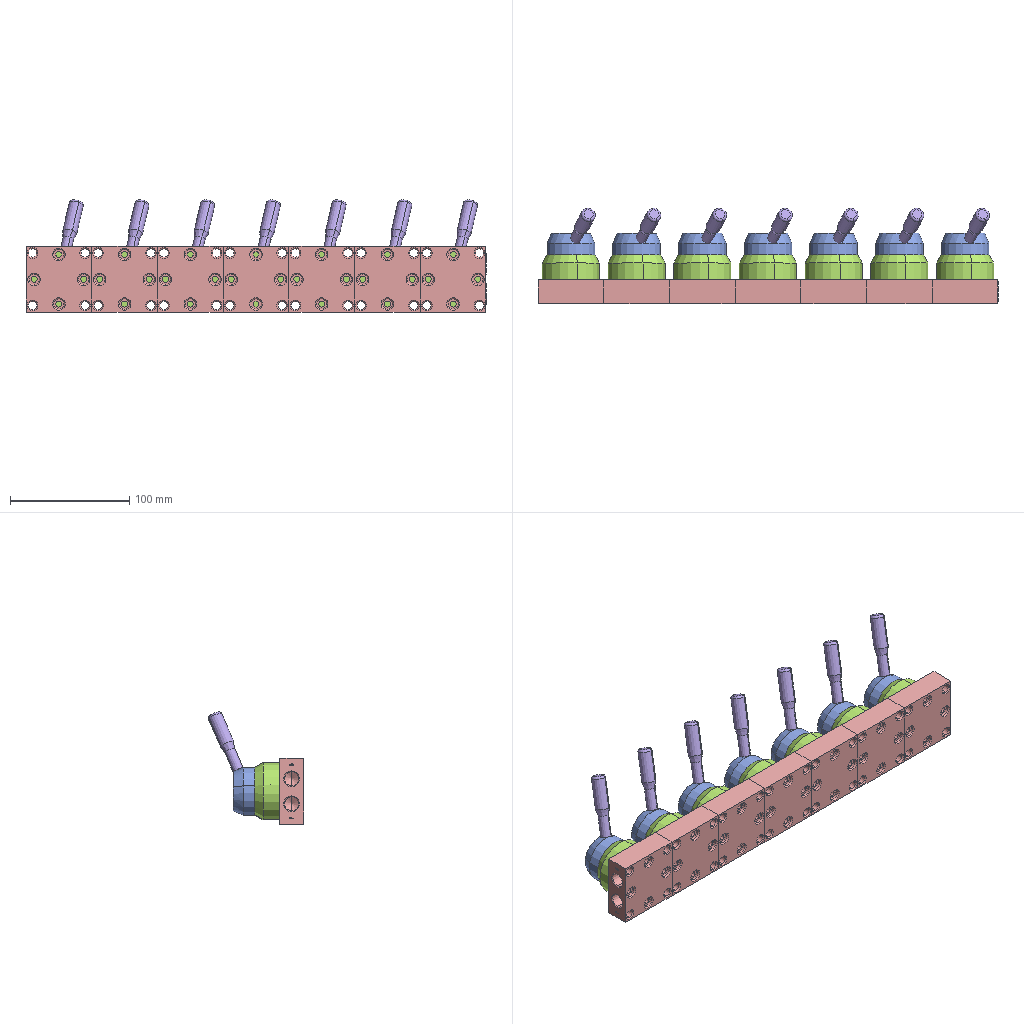Assembly | SolidWorks | 14 different items | 112 placed | box 385 x 80 x 94 mm
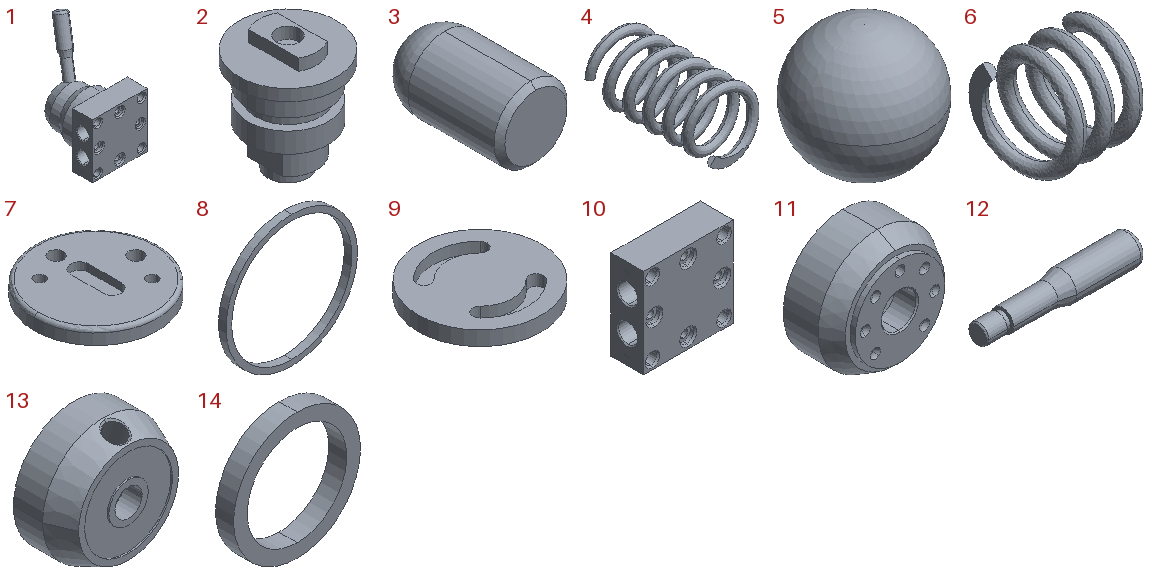Parts list (item | name | quantity | parent item | size | volume | features):
1 | (subassembly) | x7 | - | 55 x 79.723 x 94.001 mm | 101040 mm3 | features CompositeCurve 28, ReferencePattern 2, MirrorCompFeat 1
2 | - | x7 | in 1 | 17 x 17 x 19.8 mm | 2110 mm3 | features ICE 3, HoleWzd 1, Revolution 1
3 | - | x7 | in 1 | 4 x 7 x 4 mm | 79.05 mm3 | features Chamfer 1, Dome 1, Extrusion 1
4 | - | x14 | in 1 | 5.2 x 9.4 x 5.2 mm | 31.404 mm3 | features Helix 1, ICE 1, Sweep 1
5 | - | x14 | in 1 | 5.5 x 5.5 x 5.5 mm | 87.114 mm3 | features Revolution 1
6 | - | x7 | in 1 | 3 x 3.5 x 3.5 mm | 5.382 mm3 | features Helix 1, ICE 1, Sweep 1
7 | - | x7 | in 1 | 34 x 34 x 4 mm | 3323 mm3 | features ICE 2, Extrusion 1, Fillet 1
8 | - | x7 | in 1 | 35 x 2 x 35 mm | 315.73 mm3 | features Extrusion 1
9 | - | x7 | in 1 | 34 x 34 x 6 mm | 3145 mm3 | features ICE 4, Extrusion 1
10 | - | x7 | in 1 | 55 x 24 x 55 mm | 48104 mm3 | features ICE 7, MirrorPattern 4, Chamfer 2, CirPattern 2, HoleWzd 2, Extrusion 1, RefAxis 1, RevCut 1
11 | - | x7 | in 1 | 48 x 23 x 48 mm | 22097 mm3 | features ICE 4, CirPattern 2, Chamfer 1, HoleWzd 1, RevCut 1, Revolution 1
12 | - | x7 | in 1 | 62 x 12 x 12 mm | 5270 mm3 | features Chamfer 1, Fillet 1, Revolution 1
13 | - | x7 | in 1 | 40 x 18 x 40 mm | 16236 mm3 | features ICE 8, Chamfer 1, ExtruRefSurface 1, HoleWzd 1, Revolution 1
14 | - | x7 | in 1 | 14 x 2 x 14 mm | 117.81 mm3 | features Extrusion 1
Mates (type | each side: item.copy, entity, surface, feature):
In the top assembly
Coincident | 10.1 face plane Boss-Extrude1 | 10.2 face plane Boss-Extrude1 | 2 times
Coincident | 10.1 face plane Boss-Extrude1 | 10.3 face plane Boss-Extrude1 | 3 times
Coincident | 10.3 face plane Boss-Extrude1 | 10.4 face plane Boss-Extrude1 | 3 times
Coincident | 10.2 face plane Boss-Extrude1 | 10.5 face plane Boss-Extrude1 | 3 times
Coincident | 10.5 face plane Boss-Extrude1 | 10.6 face plane Boss-Extrude1
Coincident | 10.6 face plane Boss-Extrude1 | 10.7 face plane Boss-Extrude1 | 3 times
Coincident | 10.5 face plane Boss-Extrude1 | 10.7 face plane Boss-Extrude1 | 2 times
In subassembly 1
Concentric | 10.8 edge | 11.1 edge
Concentric | 10.8 edge | 13.1 edge
Concentric | 10.8 edge | 9.1 edge
Concentric | 10.8 edge | 7.1 edge
Width | 2.1 face plane Cut-Extrude2 | 2.1 face plane Cut-Extrude2 | 13.1 face plane Cut-Extrude2 | 13.1 face plane Cut-Extrude2
Coincident | 13.1 face plane Cut-Extrude1 | 2.1 face plane Revolve1
Concentric | 13.1 face cone M8 Tapped Hole1 | 12.1 edge
Tangent | 13.1 face cone Revolve1 | 12.1 face plane Revolve1
Concentric | 11.1 edge | 2.1 edge
Coincident | 5.1 face sphere Revolve1 | 4.1 select_type:24
Concentric | 13.1 edge | 11.1 edge
Concentric | 11.1 edge | 3.1 face cone Chamfer1
Coincident | 11.1 face plane Cut-Extrude3 | 3.1 face plane Boss-Extrude1
Parallel | 4.1 plane | 1.1 plane | 2 times
Coincident | 13.1 face plane Revolve1 | 11.1 face plane Revolve1
Concentric | 2.1 edge | 14.1 edge
Coincident | 2.1 edge | 14.1 edge
Coincident | 2.1 face plane Cut-Extrude3 | 6.1 face plane Cut-Extrude2
Coincident | 6.1 plane | 1.1 plane
Concentric | 2.1 edge | 6.1 select_type:24
Width | 7.1 face plane Cut-Extrude1 | 7.1 face plane Cut-Extrude1 | 2.1 face plane Cut-Extrude1 | 2.1 face plane Cut-Extrude1
Coincident | 7.1 face plane Boss-Extrude1 | 2.1 face plane Revolve1
Concentric | 7.1 edge | 9.1 edge
Coincident | 7.1 face plane Boss-Extrude1 | 9.1 face plane Boss-Extrude1
Coincident | 10.8 face plane Boss-Extrude1 | 11.1 face plane Revolve1
Concentric | 10.8 edge | 8.1 edge
Coincident | 10.8 edge | 8.1 edge
Concentric | 13.1 face cylinder Cut-Extrude4 | 5.1 face sphere Revolve1
Coincident | 13.1 face plane Cut-Extrude4 | 4.2 face plane Cut-Extrude1